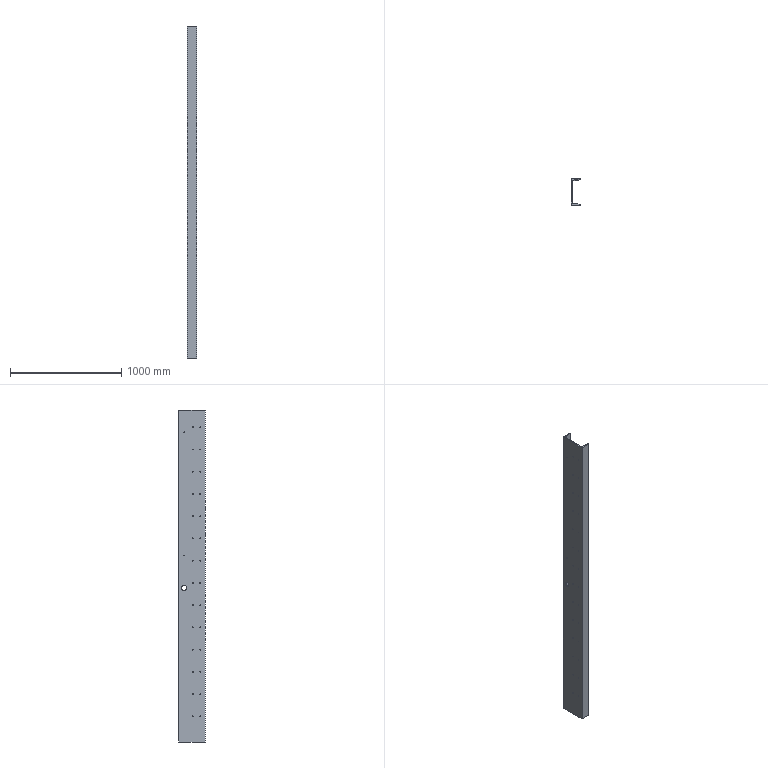Part | SolidWorks | features HoleWzd 4, Extrusion 1, ICE 1 | 1 solid | 88 faces | box 85 x 240 x 2985 mm | volume 12447040 mm3 | cylinder 77 | plane 11 | commonest cylinder face diameters 8.5 x56 6.8 x8 5 x4 10.2 x3 13 x2 26 x2